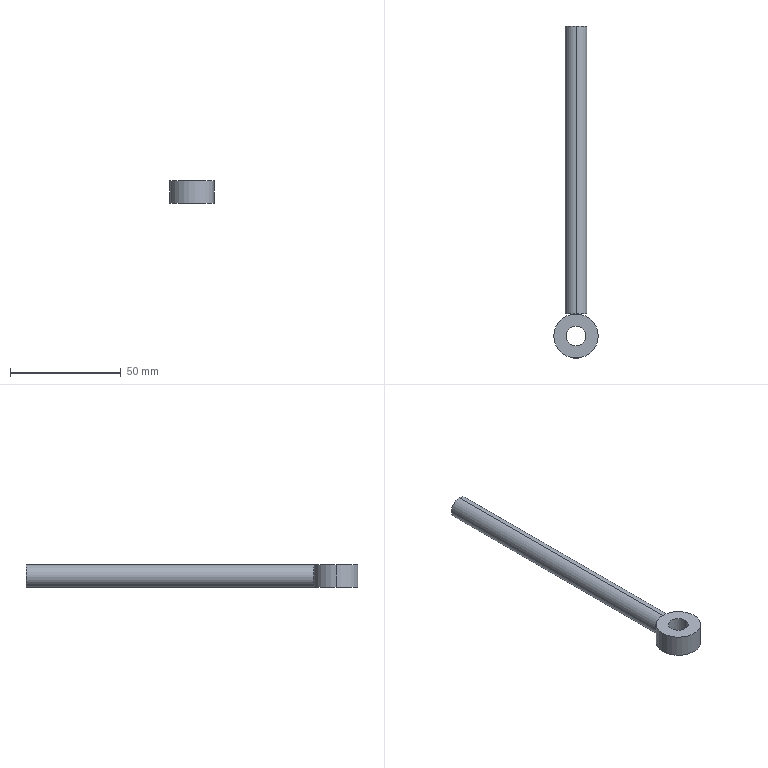Part | SolidWorks | features Extrusion 1, ICE 1, Revolution 1 | 2 solids | 10 faces | box 20 x 150 x 10 mm | volume 12716 mm3 | cylinder 6 | plane 4 | commonest cylinder face diameters 9 x2 10 x2 20 x2
STEP:
#1=CARTESIAN_POINT('',(-4.5,0.,-5.));
#2=VERTEX_POINT('',#1);
#3=CARTESIAN_POINT('',(4.5,0.,-5.));
#4=VERTEX_POINT('',#3);
#5=CARTESIAN_POINT('',(0.,0.,-5.));
#6=DIRECTION('',(0.,0.,1.));
#7=DIRECTION('',(1.,0.,0.));
#8=AXIS2_PLACEMENT_3D('',#5,#6,#7);
#9=CIRCLE('',#8,4.5);
#10=EDGE_CURVE('',#2,#4,#9,.T.);
#11=ORIENTED_EDGE('',*,*,#10,.F.);
#12=CARTESIAN_POINT('',(-4.5,0.,5.));
#13=VERTEX_POINT('',#12);
#14=CARTESIAN_POINT('',(-4.5,0.,-5.));
#15=DIRECTION('',(0.,0.,1.));
#16=VECTOR('',#15,1000.);
#17=LINE('',#14,#16);
#18=EDGE_CURVE('',#2,#13,#17,.T.);
#19=ORIENTED_EDGE('',*,*,#18,.T.);
#20=CARTESIAN_POINT('',(4.5,0.,5.));
#21=VERTEX_POINT('',#20);
#22=CARTESIAN_POINT('',(0.,0.,5.));
#23=DIRECTION('',(0.,0.,1.));
#24=DIRECTION('',(1.,0.,0.));
#25=AXIS2_PLACEMENT_3D('',#22,#23,#24);
#26=CIRCLE('',#25,4.5);
#27=EDGE_CURVE('',#13,#21,#26,.T.);
#28=ORIENTED_EDGE('',*,*,#27,.T.);
#29=CARTESIAN_POINT('',(4.5,0.,-5.));
#30=DIRECTION('',(0.,0.,1.));
#31=VECTOR('',#30,1000.);
#32=LINE('',#29,#31);
#33=EDGE_CURVE('',#4,#21,#32,.T.);
#34=ORIENTED_EDGE('',*,*,#33,.F.);
#35=EDGE_LOOP('',(#11,#19,#28,#34));
#36=FACE_OUTER_BOUND('',#35,.T.);
#37=CARTESIAN_POINT('',(0.,0.,-5.));
#38=DIRECTION('',(0.,0.,1.));
#39=DIRECTION('',(1.,0.,0.));
#40=AXIS2_PLACEMENT_3D('',#37,#38,#39);
#41=CYLINDRICAL_SURFACE('',#40,4.5);
#42=ADVANCED_FACE('',(#36),#41,.F.);
#43=CARTESIAN_POINT('',(10.,0.,5.));
#44=VERTEX_POINT('',#43);
#45=CARTESIAN_POINT('',(-10.,0.,5.));
#46=VERTEX_POINT('',#45);
#47=CARTESIAN_POINT('',(0.,0.,5.));
#48=DIRECTION('',(0.,0.,1.));
#49=DIRECTION('',(1.,0.,0.));
#50=AXIS2_PLACEMENT_3D('',#47,#48,#49);
#51=CIRCLE('',#50,10.);
#52=EDGE_CURVE('',#44,#46,#51,.T.);
#53=ORIENTED_EDGE('',*,*,#52,.F.);
#54=CARTESIAN_POINT('',(10.,0.,-5.));
#55=VERTEX_POINT('',#54);
#56=CARTESIAN_POINT('',(10.,0.,5.));
#57=DIRECTION('',(0.,0.,-1.));
#58=VECTOR('',#57,1000.);
#59=LINE('',#56,#58);
#60=EDGE_CURVE('',#44,#55,#59,.T.);
#61=ORIENTED_EDGE('',*,*,#60,.T.);
#62=CARTESIAN_POINT('',(-10.,0.,-5.));
#63=VERTEX_POINT('',#62);
#64=CARTESIAN_POINT('',(0.,0.,-5.));
#65=DIRECTION('',(0.,0.,1.));
#66=DIRECTION('',(1.,0.,0.));
#67=AXIS2_PLACEMENT_3D('',#64,#65,#66);
#68=CIRCLE('',#67,10.);
#69=EDGE_CURVE('',#55,#63,#68,.T.);
#70=ORIENTED_EDGE('',*,*,#69,.T.);
#71=CARTESIAN_POINT('',(-10.,0.,5.));
#72=DIRECTION('',(0.,0.,-1.));
#73=VECTOR('',#72,1000.);
#74=LINE('',#71,#73);
#75=EDGE_CURVE('',#46,#63,#74,.T.);
#76=ORIENTED_EDGE('',*,*,#75,.F.);
#77=EDGE_LOOP('',(#53,#61,#70,#76));
#78=FACE_OUTER_BOUND('',#77,.T.);
#79=CARTESIAN_POINT('',(0.,0.,5.));
#80=DIRECTION('',(0.,0.,-1.));
#81=DIRECTION('',(-1.,0.,0.));
#82=AXIS2_PLACEMENT_3D('',#79,#80,#81);
#83=CYLINDRICAL_SURFACE('',#82,10.);
#84=ADVANCED_FACE('',(#78),#83,.T.);
#85=ORIENTED_EDGE('',*,*,#60,.F.);
#86=CARTESIAN_POINT('',(0.,0.,5.));
#87=DIRECTION('',(0.,0.,1.));
#88=DIRECTION('',(1.,0.,0.));
#89=AXIS2_PLACEMENT_3D('',#86,#87,#88);
#90=CIRCLE('',#89,10.);
#91=EDGE_CURVE('',#46,#44,#90,.T.);
#92=ORIENTED_EDGE('',*,*,#91,.F.);
#93=ORIENTED_EDGE('',*,*,#75,.T.);
#94=CARTESIAN_POINT('',(0.,0.,-5.));
#95=DIRECTION('',(0.,0.,1.));
#96=DIRECTION('',(1.,0.,0.));
#97=AXIS2_PLACEMENT_3D('',#94,#95,#96);
#98=CIRCLE('',#97,10.);
#99=EDGE_CURVE('',#63,#55,#98,.T.);
#100=ORIENTED_EDGE('',*,*,#99,.T.);
#101=EDGE_LOOP('',(#85,#92,#93,#100));
#102=FACE_OUTER_BOUND('',#101,.T.);
#103=CARTESIAN_POINT('',(0.,0.,5.));
#104=DIRECTION('',(0.,0.,-1.));
#105=DIRECTION('',(-1.,0.,0.));
#106=AXIS2_PLACEMENT_3D('',#103,#104,#105);
#107=CYLINDRICAL_SURFACE('',#106,10.);
#108=ADVANCED_FACE('',(#102),#107,.T.);
#109=CARTESIAN_POINT('',(0.,0.,5.));
#110=DIRECTION('',(0.,0.,1.));
#111=DIRECTION('',(1.,0.,0.));
#112=AXIS2_PLACEMENT_3D('',#109,#110,#111);
#113=CIRCLE('',#112,4.5);
#114=EDGE_CURVE('',#21,#13,#113,.T.);
#115=ORIENTED_EDGE('',*,*,#114,.F.);
#116=ORIENTED_EDGE('',*,*,#27,.F.);
#117=EDGE_LOOP('',(#115,#116));
#118=FACE_BOUND('',#117,.T.);
#119=ORIENTED_EDGE('',*,*,#91,.T.);
#120=ORIENTED_EDGE('',*,*,#52,.T.);
#121=EDGE_LOOP('',(#119,#120));
#122=FACE_OUTER_BOUND('',#121,.T.);
#123=CARTESIAN_POINT('',(0.,0.,5.));
#124=DIRECTION('',(0.,0.,1.));
#125=DIRECTION('',(1.,0.,0.));
#126=AXIS2_PLACEMENT_3D('',#123,#124,#125);
#127=PLANE('',#126);
#128=ADVANCED_FACE('',(#118,#122),#127,.T.);
#129=CARTESIAN_POINT('',(0.,0.,-5.));
#130=DIRECTION('',(0.,0.,1.));
#131=DIRECTION('',(1.,0.,0.));
#132=AXIS2_PLACEMENT_3D('',#129,#130,#131);
#133=CIRCLE('',#132,4.5);
#134=EDGE_CURVE('',#4,#2,#133,.T.);
#135=ORIENTED_EDGE('',*,*,#134,.T.);
#136=ORIENTED_EDGE('',*,*,#10,.T.);
#137=EDGE_LOOP('',(#135,#136));
#138=FACE_BOUND('',#137,.T.);
#139=ORIENTED_EDGE('',*,*,#99,.F.);
#140=ORIENTED_EDGE('',*,*,#69,.F.);
#141=EDGE_LOOP('',(#139,#140));
#142=FACE_OUTER_BOUND('',#141,.T.);
#143=CARTESIAN_POINT('',(0.,0.,-5.));
#144=DIRECTION('',(0.,0.,1.));
#145=DIRECTION('',(1.,0.,0.));
#146=AXIS2_PLACEMENT_3D('',#143,#144,#145);
#147=PLANE('',#146);
#148=ADVANCED_FACE('',(#138,#142),#147,.F.);
#149=ORIENTED_EDGE('',*,*,#18,.F.);
#150=ORIENTED_EDGE('',*,*,#134,.F.);
#151=ORIENTED_EDGE('',*,*,#33,.T.);
#152=ORIENTED_EDGE('',*,*,#114,.T.);
#153=EDGE_LOOP('',(#149,#150,#151,#152));
#154=FACE_OUTER_BOUND('',#153,.T.);
#155=CARTESIAN_POINT('',(0.,0.,-5.));
#156=DIRECTION('',(0.,0.,1.));
#157=DIRECTION('',(1.,0.,0.));
#158=AXIS2_PLACEMENT_3D('',#155,#156,#157);
#159=CYLINDRICAL_SURFACE('',#158,4.5);
#160=ADVANCED_FACE('',(#154),#159,.F.);
#161=CLOSED_SHELL('',(#42,#84,#108,#128,#148,#160));
#162=MANIFOLD_SOLID_BREP('',#161);
#163=CARTESIAN_POINT('',(0.,140.,-5.));
#164=VERTEX_POINT('',#163);
#165=CARTESIAN_POINT('',(0.,140.,5.));
#166=VERTEX_POINT('',#165);
#167=CARTESIAN_POINT('',(0.,140.,0.));
#168=DIRECTION('',(0.,-1.,0.));
#169=DIRECTION('',(0.,0.,-1.));
#170=AXIS2_PLACEMENT_3D('',#167,#168,#169);
#171=CIRCLE('',#170,5.);
#172=EDGE_CURVE('',#164,#166,#171,.T.);
#173=ORIENTED_EDGE('',*,*,#172,.T.);
#174=CARTESIAN_POINT('',(0.,10.,5.));
#175=VERTEX_POINT('',#174);
#176=CARTESIAN_POINT('',(0.,10.,5.));
#177=DIRECTION('',(0.,-1.,0.));
#178=VECTOR('',#177,1000.);
#179=LINE('',#176,#178);
#180=EDGE_CURVE('',#166,#175,#179,.T.);
#181=ORIENTED_EDGE('',*,*,#180,.T.);
#182=CARTESIAN_POINT('',(0.,10.,-5.));
#183=VERTEX_POINT('',#182);
#184=CARTESIAN_POINT('',(0.,10.,0.));
#185=DIRECTION('',(0.,-1.,0.));
#186=DIRECTION('',(0.,0.,-1.));
#187=AXIS2_PLACEMENT_3D('',#184,#185,#186);
#188=CIRCLE('',#187,5.);
#189=EDGE_CURVE('',#183,#175,#188,.T.);
#190=ORIENTED_EDGE('',*,*,#189,.F.);
#191=CARTESIAN_POINT('',(0.,10.,-5.));
#192=DIRECTION('',(0.,-1.,0.));
#193=VECTOR('',#192,1000.);
#194=LINE('',#191,#193);
#195=EDGE_CURVE('',#164,#183,#194,.T.);
#196=ORIENTED_EDGE('',*,*,#195,.F.);
#197=EDGE_LOOP('',(#173,#181,#190,#196));
#198=FACE_OUTER_BOUND('',#197,.T.);
#199=CARTESIAN_POINT('',(0.,10.,0.));
#200=DIRECTION('',(0.,-1.,0.));
#201=DIRECTION('',(0.,0.,-1.));
#202=AXIS2_PLACEMENT_3D('',#199,#200,#201);
#203=CYLINDRICAL_SURFACE('',#202,5.);
#204=ADVANCED_FACE('',(#198),#203,.T.);
#205=ORIENTED_EDGE('',*,*,#189,.T.);
#206=CARTESIAN_POINT('',(0.,10.,0.));
#207=DIRECTION('',(0.,-1.,0.));
#208=DIRECTION('',(0.,0.,-1.));
#209=AXIS2_PLACEMENT_3D('',#206,#207,#208);
#210=CIRCLE('',#209,5.);
#211=EDGE_CURVE('',#175,#183,#210,.T.);
#212=ORIENTED_EDGE('',*,*,#211,.T.);
#213=EDGE_LOOP('',(#205,#212));
#214=FACE_OUTER_BOUND('',#213,.T.);
#215=CARTESIAN_POINT('',(5.,10.,0.));
#216=DIRECTION('',(0.,-1.,0.));
#217=DIRECTION('',(0.,0.,-1.));
#218=AXIS2_PLACEMENT_3D('',#215,#216,#217);
#219=PLANE('',#218);
#220=ADVANCED_FACE('',(#214),#219,.T.);
#221=ORIENTED_EDGE('',*,*,#172,.F.);
#222=CARTESIAN_POINT('',(0.,140.,0.));
#223=DIRECTION('',(0.,-1.,0.));
#224=DIRECTION('',(0.,0.,-1.));
#225=AXIS2_PLACEMENT_3D('',#222,#223,#224);
#226=CIRCLE('',#225,5.);
#227=EDGE_CURVE('',#166,#164,#226,.T.);
#228=ORIENTED_EDGE('',*,*,#227,.F.);
#229=EDGE_LOOP('',(#221,#228));
#230=FACE_OUTER_BOUND('',#229,.T.);
#231=CARTESIAN_POINT('',(0.,140.,0.));
#232=DIRECTION('',(0.,1.,0.));
#233=DIRECTION('',(0.,0.,1.));
#234=AXIS2_PLACEMENT_3D('',#231,#232,#233);
#235=PLANE('',#234);
#236=ADVANCED_FACE('',(#230),#235,.T.);
#237=ORIENTED_EDGE('',*,*,#180,.F.);
#238=ORIENTED_EDGE('',*,*,#227,.T.);
#239=ORIENTED_EDGE('',*,*,#195,.T.);
#240=ORIENTED_EDGE('',*,*,#211,.F.);
#241=EDGE_LOOP('',(#237,#238,#239,#240));
#242=FACE_OUTER_BOUND('',#241,.T.);
#243=CARTESIAN_POINT('',(0.,10.,0.));
#244=DIRECTION('',(0.,-1.,0.));
#245=DIRECTION('',(0.,0.,-1.));
#246=AXIS2_PLACEMENT_3D('',#243,#244,#245);
#247=CYLINDRICAL_SURFACE('',#246,5.);
#248=ADVANCED_FACE('',(#242),#247,.T.);
#249=CLOSED_SHELL('',(#204,#220,#236,#248));
#250=MANIFOLD_SOLID_BREP('',#249);
#251=CARTESIAN_POINT('',(0.,0.,0.));
#252=DIRECTION('',(0.,0.,1.));
#253=DIRECTION('',(1.,0.,0.));
#254=AXIS2_PLACEMENT_3D('',#251,#252,#253);
#255=(LENGTH_UNIT()NAMED_UNIT(*)SI_UNIT(.MILLI.,.METRE.));
#256=UNCERTAINTY_MEASURE_WITH_UNIT(LENGTH_MEASURE(0.00001),#255,'','');
#257=(NAMED_UNIT(*)PLANE_ANGLE_UNIT()SI_UNIT($,.RADIAN.));
#258=(NAMED_UNIT(*)SI_UNIT($,.STERADIAN.)SOLID_ANGLE_UNIT());
#259=(GEOMETRIC_REPRESENTATION_CONTEXT(3)GLOBAL_UNCERTAINTY_ASSIGNED_CONTEXT((#256))GLOBAL_UNIT_ASSIGNED_CONTEXT((#255,#257,#258))REPRESENTATION_CONTEXT('',''));
#260=ADVANCED_BREP_SHAPE_REPRESENTATION('',(#162,#250,#254),#259);